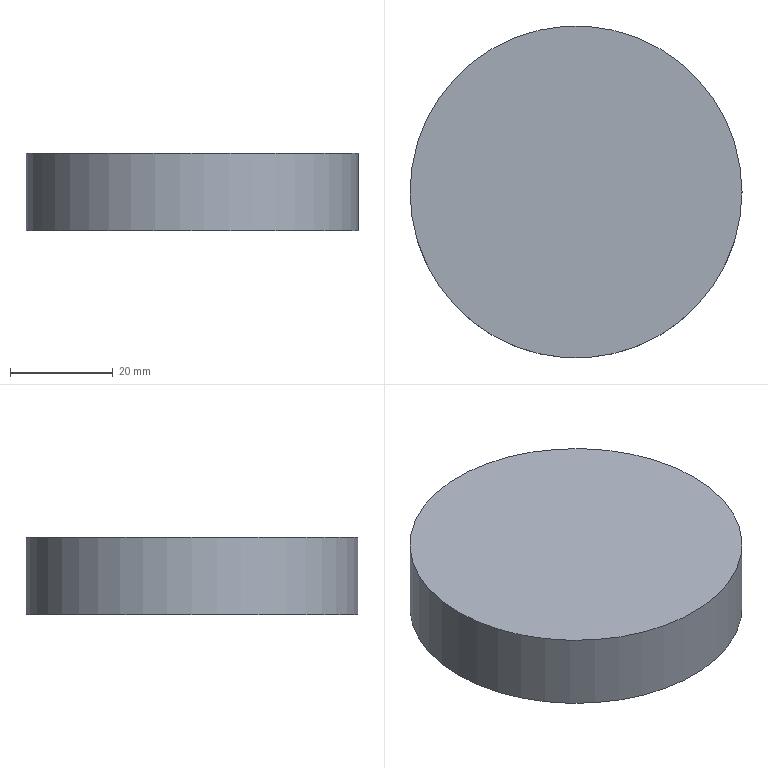Part | NX | features solid 2 | 1 solid | 3 faces | box 64.492 x 64.492 x 15 mm | volume 49000 mm3 | plane 2 | cylinder 1 | commonest cylinder face diameters 64.492 x1
STEP:
#1=CARTESIAN_POINT('',(-47.754,-440.,-196.));
#2=VERTEX_POINT('',#1);
#3=CARTESIAN_POINT('',(-80.,-440.,-196.));
#4=DIRECTION('',(0.,0.,1.));
#5=DIRECTION('',(1.,0.,0.));
#6=AXIS2_PLACEMENT_3D('',#3,#4,#5);
#7=CIRCLE('',#6,32.246);
#8=EDGE_CURVE('',#2,#2,#7,.T.);
#9=ORIENTED_EDGE('',*,*,#8,.T.);
#10=EDGE_LOOP('',(#9));
#11=FACE_BOUND('',#10,.T.);
#12=CARTESIAN_POINT('',(-47.754,-440.,-181.));
#13=VERTEX_POINT('',#12);
#14=CARTESIAN_POINT('',(-80.,-440.,-181.));
#15=DIRECTION('',(0.,0.,1.));
#16=DIRECTION('',(1.,0.,0.));
#17=AXIS2_PLACEMENT_3D('',#14,#15,#16);
#18=CIRCLE('',#17,32.246);
#19=EDGE_CURVE('',#13,#13,#18,.T.);
#20=ORIENTED_EDGE('',*,*,#19,.F.);
#21=EDGE_LOOP('',(#20));
#22=FACE_BOUND('',#21,.T.);
#23=CARTESIAN_POINT('',(-80.,-440.,-196.));
#24=DIRECTION('',(0.,0.,1.));
#25=DIRECTION('',(-1.,0.,0.));
#26=AXIS2_PLACEMENT_3D('',#23,#24,#25);
#27=CYLINDRICAL_SURFACE('',#26,32.246);
#28=ADVANCED_FACE('',(#11,#22),#27,.T.);
#29=ORIENTED_EDGE('',*,*,#8,.F.);
#30=EDGE_LOOP('',(#29));
#31=FACE_BOUND('',#30,.T.);
#32=CARTESIAN_POINT('',(-80.,-440.,-196.));
#33=DIRECTION('',(0.,0.,-1.));
#34=DIRECTION('',(1.,0.,0.));
#35=AXIS2_PLACEMENT_3D('',#32,#33,#34);
#36=PLANE('',#35);
#37=ADVANCED_FACE('',(#31),#36,.T.);
#38=ORIENTED_EDGE('',*,*,#19,.T.);
#39=EDGE_LOOP('',(#38));
#40=FACE_BOUND('',#39,.T.);
#41=CARTESIAN_POINT('',(-80.,-440.,-181.));
#42=DIRECTION('',(0.,0.,-1.));
#43=DIRECTION('',(1.,0.,0.));
#44=AXIS2_PLACEMENT_3D('',#41,#42,#43);
#45=PLANE('',#44);
#46=ADVANCED_FACE('',(#40),#45,.F.);
#47=CLOSED_SHELL('',(#28,#37,#46));
#48=MANIFOLD_SOLID_BREP('',#47);
#49=(LENGTH_UNIT()NAMED_UNIT(*)SI_UNIT(.MILLI.,.METRE.));
#50=UNCERTAINTY_MEASURE_WITH_UNIT(LENGTH_MEASURE(0.00001),#49,'','');
#51=(NAMED_UNIT(*)PLANE_ANGLE_UNIT()SI_UNIT($,.RADIAN.));
#52=(NAMED_UNIT(*)SI_UNIT($,.STERADIAN.)SOLID_ANGLE_UNIT());
#53=(GEOMETRIC_REPRESENTATION_CONTEXT(3)GLOBAL_UNCERTAINTY_ASSIGNED_CONTEXT((#50))GLOBAL_UNIT_ASSIGNED_CONTEXT((#49,#51,#52))REPRESENTATION_CONTEXT('',''));
#54=ADVANCED_BREP_SHAPE_REPRESENTATION('',(#48),#53);